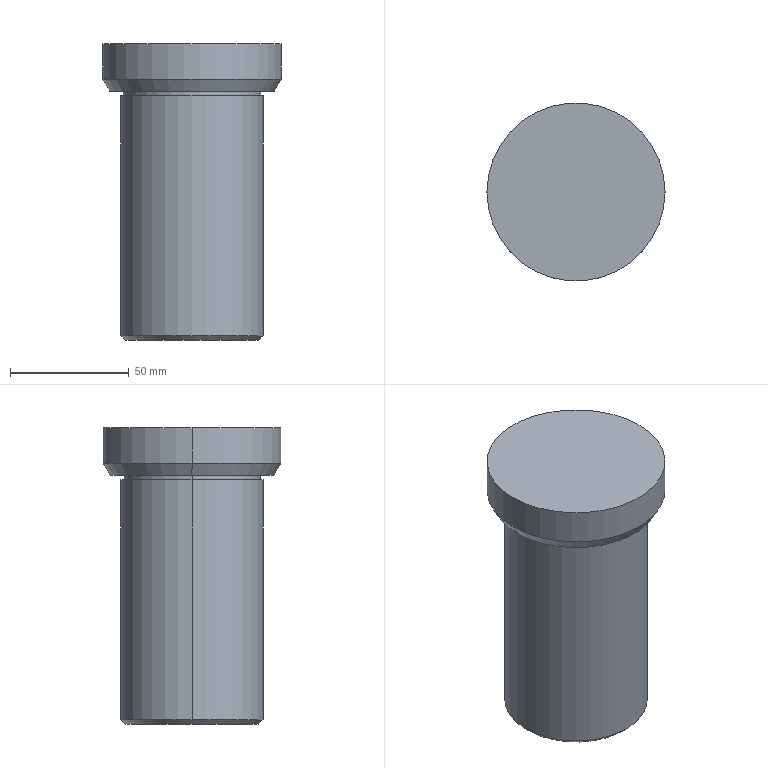Part | SolidWorks | features Chamfer 2, Extrusion 1, ICE 1, RefAxis 1, RevCut 1 | 1 solid | 14 faces | box 75 x 75 x 125 mm | volume 382842 mm3 | cylinder 6 | cone 4 | plane 4 | commonest cylinder face diameters 58 x2 60 x2 75 x2
STEP:
#1=CARTESIAN_POINT('',(-34.613,0.,105.));
#2=VERTEX_POINT('',#1);
#3=CARTESIAN_POINT('',(34.613,0.,105.));
#4=VERTEX_POINT('',#3);
#5=CARTESIAN_POINT('',(0.,0.,105.));
#6=DIRECTION('',(0.,0.,-1.));
#7=DIRECTION('',(1.,0.,0.));
#8=AXIS2_PLACEMENT_3D('',#5,#6,#7);
#9=CIRCLE('',#8,34.613);
#10=EDGE_CURVE('',#2,#4,#9,.T.);
#11=ORIENTED_EDGE('',*,*,#10,.F.);
#12=CARTESIAN_POINT('',(-37.5,0.,110.));
#13=VERTEX_POINT('',#12);
#14=CARTESIAN_POINT('',(-37.5,0.,110.));
#15=DIRECTION('',(-0.5,0.,0.866));
#16=VECTOR('',#15,1000.);
#17=LINE('',#14,#16);
#18=EDGE_CURVE('',#2,#13,#17,.T.);
#19=ORIENTED_EDGE('',*,*,#18,.T.);
#20=CARTESIAN_POINT('',(37.5,0.,110.));
#21=VERTEX_POINT('',#20);
#22=CARTESIAN_POINT('',(0.,0.,110.));
#23=DIRECTION('',(0.,0.,1.));
#24=DIRECTION('',(1.,0.,0.));
#25=AXIS2_PLACEMENT_3D('',#22,#23,#24);
#26=CIRCLE('',#25,37.5);
#27=EDGE_CURVE('',#21,#13,#26,.T.);
#28=ORIENTED_EDGE('',*,*,#27,.F.);
#29=CARTESIAN_POINT('',(37.5,0.,110.));
#30=DIRECTION('',(0.5,0.,0.866));
#31=VECTOR('',#30,1000.);
#32=LINE('',#29,#31);
#33=EDGE_CURVE('',#4,#21,#32,.T.);
#34=ORIENTED_EDGE('',*,*,#33,.F.);
#35=EDGE_LOOP('',(#11,#19,#28,#34));
#36=FACE_OUTER_BOUND('',#35,.T.);
#37=CARTESIAN_POINT('',(0.,0.,110.));
#38=DIRECTION('',(0.,0.,1.));
#39=DIRECTION('',(1.,0.,0.));
#40=AXIS2_PLACEMENT_3D('',#37,#38,#39);
#41=CONICAL_SURFACE('',#40,37.5,0.5236);
#42=ADVANCED_FACE('',(#36),#41,.T.);
#43=CARTESIAN_POINT('',(37.5,0.,125.));
#44=VERTEX_POINT('',#43);
#45=CARTESIAN_POINT('',(-37.5,0.,125.));
#46=VERTEX_POINT('',#45);
#47=CARTESIAN_POINT('',(0.,0.,125.));
#48=DIRECTION('',(0.,0.,1.));
#49=DIRECTION('',(1.,0.,0.));
#50=AXIS2_PLACEMENT_3D('',#47,#48,#49);
#51=CIRCLE('',#50,37.5);
#52=EDGE_CURVE('',#44,#46,#51,.T.);
#53=ORIENTED_EDGE('',*,*,#52,.F.);
#54=CARTESIAN_POINT('',(37.5,0.,125.));
#55=DIRECTION('',(0.,0.,-1.));
#56=VECTOR('',#55,1000.);
#57=LINE('',#54,#56);
#58=EDGE_CURVE('',#44,#21,#57,.T.);
#59=ORIENTED_EDGE('',*,*,#58,.T.);
#60=ORIENTED_EDGE('',*,*,#27,.T.);
#61=CARTESIAN_POINT('',(-37.5,0.,125.));
#62=DIRECTION('',(0.,0.,-1.));
#63=VECTOR('',#62,1000.);
#64=LINE('',#61,#63);
#65=EDGE_CURVE('',#46,#13,#64,.T.);
#66=ORIENTED_EDGE('',*,*,#65,.F.);
#67=EDGE_LOOP('',(#53,#59,#60,#66));
#68=FACE_OUTER_BOUND('',#67,.T.);
#69=CARTESIAN_POINT('',(0.,0.,125.));
#70=DIRECTION('',(0.,0.,-1.));
#71=DIRECTION('',(-1.,0.,0.));
#72=AXIS2_PLACEMENT_3D('',#69,#70,#71);
#73=CYLINDRICAL_SURFACE('',#72,37.5);
#74=ADVANCED_FACE('',(#68),#73,.T.);
#75=CARTESIAN_POINT('',(29.,0.,103.));
#76=VERTEX_POINT('',#75);
#77=CARTESIAN_POINT('',(-29.,0.,103.));
#78=VERTEX_POINT('',#77);
#79=CARTESIAN_POINT('',(0.,0.,103.));
#80=DIRECTION('',(0.,0.,1.));
#81=DIRECTION('',(1.,0.,0.));
#82=AXIS2_PLACEMENT_3D('',#79,#80,#81);
#83=CIRCLE('',#82,29.);
#84=EDGE_CURVE('',#76,#78,#83,.T.);
#85=ORIENTED_EDGE('',*,*,#84,.T.);
#86=CARTESIAN_POINT('',(-29.,0.,105.));
#87=VERTEX_POINT('',#86);
#88=CARTESIAN_POINT('',(-29.,0.,105.));
#89=DIRECTION('',(0.,0.,1.));
#90=VECTOR('',#89,1000.);
#91=LINE('',#88,#90);
#92=EDGE_CURVE('',#78,#87,#91,.T.);
#93=ORIENTED_EDGE('',*,*,#92,.T.);
#94=CARTESIAN_POINT('',(29.,0.,105.));
#95=VERTEX_POINT('',#94);
#96=CARTESIAN_POINT('',(0.,0.,105.));
#97=DIRECTION('',(0.,0.,1.));
#98=DIRECTION('',(1.,0.,0.));
#99=AXIS2_PLACEMENT_3D('',#96,#97,#98);
#100=CIRCLE('',#99,29.);
#101=EDGE_CURVE('',#95,#87,#100,.T.);
#102=ORIENTED_EDGE('',*,*,#101,.F.);
#103=CARTESIAN_POINT('',(29.,0.,105.));
#104=DIRECTION('',(0.,0.,1.));
#105=VECTOR('',#104,1000.);
#106=LINE('',#103,#105);
#107=EDGE_CURVE('',#76,#95,#106,.T.);
#108=ORIENTED_EDGE('',*,*,#107,.F.);
#109=EDGE_LOOP('',(#85,#93,#102,#108));
#110=FACE_OUTER_BOUND('',#109,.T.);
#111=CARTESIAN_POINT('',(0.,0.,105.));
#112=DIRECTION('',(0.,0.,1.));
#113=DIRECTION('',(1.,0.,0.));
#114=AXIS2_PLACEMENT_3D('',#111,#112,#113);
#115=CYLINDRICAL_SURFACE('',#114,29.);
#116=ADVANCED_FACE('',(#110),#115,.T.);
#117=CARTESIAN_POINT('',(-28.,0.,0.));
#118=VERTEX_POINT('',#117);
#119=CARTESIAN_POINT('',(28.,0.,0.));
#120=VERTEX_POINT('',#119);
#121=CARTESIAN_POINT('',(0.,0.,0.));
#122=DIRECTION('',(0.,0.,-1.));
#123=DIRECTION('',(1.,0.,0.));
#124=AXIS2_PLACEMENT_3D('',#121,#122,#123);
#125=CIRCLE('',#124,28.);
#126=EDGE_CURVE('',#118,#120,#125,.T.);
#127=ORIENTED_EDGE('',*,*,#126,.F.);
#128=CARTESIAN_POINT('',(-30.,0.,2.));
#129=VERTEX_POINT('',#128);
#130=CARTESIAN_POINT('',(-30.,0.,2.));
#131=DIRECTION('',(-0.7071,0.,0.7071));
#132=VECTOR('',#131,1000.);
#133=LINE('',#130,#132);
#134=EDGE_CURVE('',#118,#129,#133,.T.);
#135=ORIENTED_EDGE('',*,*,#134,.T.);
#136=CARTESIAN_POINT('',(30.,0.,2.));
#137=VERTEX_POINT('',#136);
#138=CARTESIAN_POINT('',(0.,0.,2.));
#139=DIRECTION('',(0.,0.,1.));
#140=DIRECTION('',(1.,0.,0.));
#141=AXIS2_PLACEMENT_3D('',#138,#139,#140);
#142=CIRCLE('',#141,30.);
#143=EDGE_CURVE('',#137,#129,#142,.T.);
#144=ORIENTED_EDGE('',*,*,#143,.F.);
#145=CARTESIAN_POINT('',(30.,0.,2.));
#146=DIRECTION('',(0.7071,0.,0.7071));
#147=VECTOR('',#146,1000.);
#148=LINE('',#145,#147);
#149=EDGE_CURVE('',#120,#137,#148,.T.);
#150=ORIENTED_EDGE('',*,*,#149,.F.);
#151=EDGE_LOOP('',(#127,#135,#144,#150));
#152=FACE_OUTER_BOUND('',#151,.T.);
#153=CARTESIAN_POINT('',(0.,0.,2.));
#154=DIRECTION('',(0.,0.,1.));
#155=DIRECTION('',(1.,0.,0.));
#156=AXIS2_PLACEMENT_3D('',#153,#154,#155);
#157=CONICAL_SURFACE('',#156,30.,0.7854);
#158=ADVANCED_FACE('',(#152),#157,.T.);
#159=CARTESIAN_POINT('',(30.,0.,103.));
#160=VERTEX_POINT('',#159);
#161=CARTESIAN_POINT('',(-30.,0.,103.));
#162=VERTEX_POINT('',#161);
#163=CARTESIAN_POINT('',(0.,0.,103.));
#164=DIRECTION('',(0.,0.,1.));
#165=DIRECTION('',(1.,0.,0.));
#166=AXIS2_PLACEMENT_3D('',#163,#164,#165);
#167=CIRCLE('',#166,30.);
#168=EDGE_CURVE('',#160,#162,#167,.T.);
#169=ORIENTED_EDGE('',*,*,#168,.F.);
#170=CARTESIAN_POINT('',(30.,0.,105.));
#171=DIRECTION('',(0.,0.,-1.));
#172=VECTOR('',#171,1000.);
#173=LINE('',#170,#172);
#174=EDGE_CURVE('',#160,#137,#173,.T.);
#175=ORIENTED_EDGE('',*,*,#174,.T.);
#176=ORIENTED_EDGE('',*,*,#143,.T.);
#177=CARTESIAN_POINT('',(-30.,0.,105.));
#178=DIRECTION('',(0.,0.,-1.));
#179=VECTOR('',#178,1000.);
#180=LINE('',#177,#179);
#181=EDGE_CURVE('',#162,#129,#180,.T.);
#182=ORIENTED_EDGE('',*,*,#181,.F.);
#183=EDGE_LOOP('',(#169,#175,#176,#182));
#184=FACE_OUTER_BOUND('',#183,.T.);
#185=CARTESIAN_POINT('',(0.,0.,105.));
#186=DIRECTION('',(0.,0.,-1.));
#187=DIRECTION('',(-1.,0.,0.));
#188=AXIS2_PLACEMENT_3D('',#185,#186,#187);
#189=CYLINDRICAL_SURFACE('',#188,30.);
#190=ADVANCED_FACE('',(#184),#189,.T.);
#191=ORIENTED_EDGE('',*,*,#174,.F.);
#192=CARTESIAN_POINT('',(0.,0.,103.));
#193=DIRECTION('',(0.,0.,1.));
#194=DIRECTION('',(1.,0.,0.));
#195=AXIS2_PLACEMENT_3D('',#192,#193,#194);
#196=CIRCLE('',#195,30.);
#197=EDGE_CURVE('',#162,#160,#196,.T.);
#198=ORIENTED_EDGE('',*,*,#197,.F.);
#199=ORIENTED_EDGE('',*,*,#181,.T.);
#200=CARTESIAN_POINT('',(0.,0.,2.));
#201=DIRECTION('',(0.,0.,1.));
#202=DIRECTION('',(1.,0.,0.));
#203=AXIS2_PLACEMENT_3D('',#200,#201,#202);
#204=CIRCLE('',#203,30.);
#205=EDGE_CURVE('',#129,#137,#204,.T.);
#206=ORIENTED_EDGE('',*,*,#205,.T.);
#207=EDGE_LOOP('',(#191,#198,#199,#206));
#208=FACE_OUTER_BOUND('',#207,.T.);
#209=CARTESIAN_POINT('',(0.,0.,105.));
#210=DIRECTION('',(0.,0.,-1.));
#211=DIRECTION('',(-1.,0.,0.));
#212=AXIS2_PLACEMENT_3D('',#209,#210,#211);
#213=CYLINDRICAL_SURFACE('',#212,30.);
#214=ADVANCED_FACE('',(#208),#213,.T.);
#215=CARTESIAN_POINT('',(0.,0.,0.));
#216=DIRECTION('',(0.,0.,-1.));
#217=DIRECTION('',(1.,0.,0.));
#218=AXIS2_PLACEMENT_3D('',#215,#216,#217);
#219=CIRCLE('',#218,28.);
#220=EDGE_CURVE('',#120,#118,#219,.T.);
#221=ORIENTED_EDGE('',*,*,#220,.T.);
#222=ORIENTED_EDGE('',*,*,#126,.T.);
#223=EDGE_LOOP('',(#221,#222));
#224=FACE_OUTER_BOUND('',#223,.T.);
#225=CARTESIAN_POINT('',(0.,0.,0.));
#226=DIRECTION('',(0.,0.,1.));
#227=DIRECTION('',(1.,0.,0.));
#228=AXIS2_PLACEMENT_3D('',#225,#226,#227);
#229=PLANE('',#228);
#230=ADVANCED_FACE('',(#224),#229,.F.);
#231=ORIENTED_EDGE('',*,*,#134,.F.);
#232=ORIENTED_EDGE('',*,*,#220,.F.);
#233=ORIENTED_EDGE('',*,*,#149,.T.);
#234=ORIENTED_EDGE('',*,*,#205,.F.);
#235=EDGE_LOOP('',(#231,#232,#233,#234));
#236=FACE_OUTER_BOUND('',#235,.T.);
#237=CARTESIAN_POINT('',(0.,0.,2.));
#238=DIRECTION('',(0.,0.,1.));
#239=DIRECTION('',(1.,0.,0.));
#240=AXIS2_PLACEMENT_3D('',#237,#238,#239);
#241=CONICAL_SURFACE('',#240,30.,0.7854);
#242=ADVANCED_FACE('',(#236),#241,.T.);
#243=ORIENTED_EDGE('',*,*,#84,.F.);
#244=CARTESIAN_POINT('',(0.,0.,103.));
#245=DIRECTION('',(0.,0.,1.));
#246=DIRECTION('',(1.,0.,0.));
#247=AXIS2_PLACEMENT_3D('',#244,#245,#246);
#248=CIRCLE('',#247,29.);
#249=EDGE_CURVE('',#78,#76,#248,.T.);
#250=ORIENTED_EDGE('',*,*,#249,.F.);
#251=EDGE_LOOP('',(#243,#250));
#252=FACE_BOUND('',#251,.T.);
#253=ORIENTED_EDGE('',*,*,#197,.T.);
#254=ORIENTED_EDGE('',*,*,#168,.T.);
#255=EDGE_LOOP('',(#253,#254));
#256=FACE_OUTER_BOUND('',#255,.T.);
#257=CARTESIAN_POINT('',(30.,0.,103.));
#258=DIRECTION('',(0.,0.,-1.));
#259=DIRECTION('',(-1.,0.,0.));
#260=AXIS2_PLACEMENT_3D('',#257,#258,#259);
#261=PLANE('',#260);
#262=ADVANCED_FACE('',(#252,#256),#261,.F.);
#263=ORIENTED_EDGE('',*,*,#92,.F.);
#264=ORIENTED_EDGE('',*,*,#249,.T.);
#265=ORIENTED_EDGE('',*,*,#107,.T.);
#266=CARTESIAN_POINT('',(0.,0.,105.));
#267=DIRECTION('',(0.,0.,1.));
#268=DIRECTION('',(1.,0.,0.));
#269=AXIS2_PLACEMENT_3D('',#266,#267,#268);
#270=CIRCLE('',#269,29.);
#271=EDGE_CURVE('',#87,#95,#270,.T.);
#272=ORIENTED_EDGE('',*,*,#271,.F.);
#273=EDGE_LOOP('',(#263,#264,#265,#272));
#274=FACE_OUTER_BOUND('',#273,.T.);
#275=CARTESIAN_POINT('',(0.,0.,105.));
#276=DIRECTION('',(0.,0.,1.));
#277=DIRECTION('',(1.,0.,0.));
#278=AXIS2_PLACEMENT_3D('',#275,#276,#277);
#279=CYLINDRICAL_SURFACE('',#278,29.);
#280=ADVANCED_FACE('',(#274),#279,.T.);
#281=CARTESIAN_POINT('',(0.,0.,125.));
#282=DIRECTION('',(0.,0.,1.));
#283=DIRECTION('',(1.,0.,0.));
#284=AXIS2_PLACEMENT_3D('',#281,#282,#283);
#285=CIRCLE('',#284,37.5);
#286=EDGE_CURVE('',#46,#44,#285,.T.);
#287=ORIENTED_EDGE('',*,*,#286,.T.);
#288=ORIENTED_EDGE('',*,*,#52,.T.);
#289=EDGE_LOOP('',(#287,#288));
#290=FACE_OUTER_BOUND('',#289,.T.);
#291=CARTESIAN_POINT('',(0.,0.,125.));
#292=DIRECTION('',(0.,0.,1.));
#293=DIRECTION('',(1.,0.,0.));
#294=AXIS2_PLACEMENT_3D('',#291,#292,#293);
#295=PLANE('',#294);
#296=ADVANCED_FACE('',(#290),#295,.T.);
#297=ORIENTED_EDGE('',*,*,#58,.F.);
#298=ORIENTED_EDGE('',*,*,#286,.F.);
#299=ORIENTED_EDGE('',*,*,#65,.T.);
#300=CARTESIAN_POINT('',(0.,0.,110.));
#301=DIRECTION('',(0.,0.,1.));
#302=DIRECTION('',(1.,0.,0.));
#303=AXIS2_PLACEMENT_3D('',#300,#301,#302);
#304=CIRCLE('',#303,37.5);
#305=EDGE_CURVE('',#13,#21,#304,.T.);
#306=ORIENTED_EDGE('',*,*,#305,.T.);
#307=EDGE_LOOP('',(#297,#298,#299,#306));
#308=FACE_OUTER_BOUND('',#307,.T.);
#309=CARTESIAN_POINT('',(0.,0.,125.));
#310=DIRECTION('',(0.,0.,-1.));
#311=DIRECTION('',(-1.,0.,0.));
#312=AXIS2_PLACEMENT_3D('',#309,#310,#311);
#313=CYLINDRICAL_SURFACE('',#312,37.5);
#314=ADVANCED_FACE('',(#308),#313,.T.);
#315=CARTESIAN_POINT('',(0.,0.,105.));
#316=DIRECTION('',(0.,0.,-1.));
#317=DIRECTION('',(1.,0.,0.));
#318=AXIS2_PLACEMENT_3D('',#315,#316,#317);
#319=CIRCLE('',#318,34.613);
#320=EDGE_CURVE('',#4,#2,#319,.T.);
#321=ORIENTED_EDGE('',*,*,#320,.T.);
#322=ORIENTED_EDGE('',*,*,#10,.T.);
#323=EDGE_LOOP('',(#321,#322));
#324=FACE_OUTER_BOUND('',#323,.T.);
#325=ORIENTED_EDGE('',*,*,#101,.T.);
#326=ORIENTED_EDGE('',*,*,#271,.T.);
#327=EDGE_LOOP('',(#325,#326));
#328=FACE_BOUND('',#327,.T.);
#329=CARTESIAN_POINT('',(0.,0.,105.));
#330=DIRECTION('',(0.,0.,1.));
#331=DIRECTION('',(1.,0.,0.));
#332=AXIS2_PLACEMENT_3D('',#329,#330,#331);
#333=PLANE('',#332);
#334=ADVANCED_FACE('',(#324,#328),#333,.F.);
#335=ORIENTED_EDGE('',*,*,#18,.F.);
#336=ORIENTED_EDGE('',*,*,#320,.F.);
#337=ORIENTED_EDGE('',*,*,#33,.T.);
#338=ORIENTED_EDGE('',*,*,#305,.F.);
#339=EDGE_LOOP('',(#335,#336,#337,#338));
#340=FACE_OUTER_BOUND('',#339,.T.);
#341=CARTESIAN_POINT('',(0.,0.,110.));
#342=DIRECTION('',(0.,0.,1.));
#343=DIRECTION('',(1.,0.,0.));
#344=AXIS2_PLACEMENT_3D('',#341,#342,#343);
#345=CONICAL_SURFACE('',#344,37.5,0.5236);
#346=ADVANCED_FACE('',(#340),#345,.T.);
#347=CLOSED_SHELL('',(#42,#74,#116,#158,#190,#214,#230,#242,#262,#280,#296,#314,#334,#346));
#348=MANIFOLD_SOLID_BREP('',#347);
#349=CARTESIAN_POINT('',(0.,0.,0.));
#350=DIRECTION('',(0.,0.,1.));
#351=DIRECTION('',(1.,0.,0.));
#352=AXIS2_PLACEMENT_3D('',#349,#350,#351);
#353=(LENGTH_UNIT()NAMED_UNIT(*)SI_UNIT(.MILLI.,.METRE.));
#354=UNCERTAINTY_MEASURE_WITH_UNIT(LENGTH_MEASURE(0.00001),#353,'','');
#355=(NAMED_UNIT(*)PLANE_ANGLE_UNIT()SI_UNIT($,.RADIAN.));
#356=(NAMED_UNIT(*)SI_UNIT($,.STERADIAN.)SOLID_ANGLE_UNIT());
#357=(GEOMETRIC_REPRESENTATION_CONTEXT(3)GLOBAL_UNCERTAINTY_ASSIGNED_CONTEXT((#354))GLOBAL_UNIT_ASSIGNED_CONTEXT((#353,#355,#356))REPRESENTATION_CONTEXT('',''));
#358=ADVANCED_BREP_SHAPE_REPRESENTATION('',(#348,#352),#357);